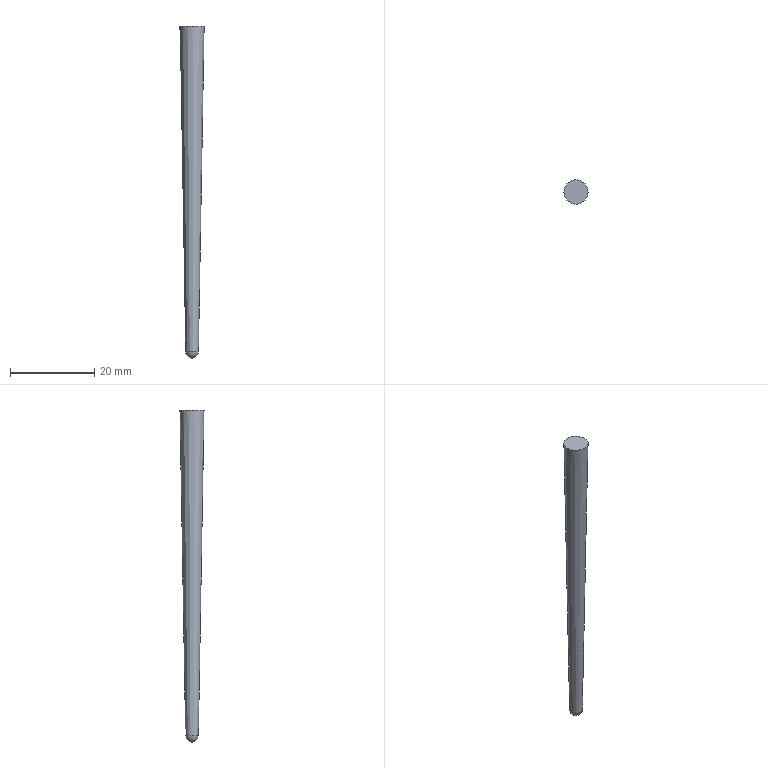Part | NX | features solid 2 | 1 solid | 4 faces | box 5.751 x 5.751 x 78.8 mm | volume 1220 mm3 | plane 2 | cone 1 | torus 1
STEP:
#1=CARTESIAN_POINT('',(-0.02595,0.,23.24));
#2=VERTEX_POINT('',#1);
#3=CARTESIAN_POINT('',(0.,0.,23.24));
#4=DIRECTION('',(0.,0.,-1.));
#5=DIRECTION('',(-1.,0.,0.));
#6=AXIS2_PLACEMENT_3D('',#3,#4,#5);
#7=CIRCLE('',#6,0.02595);
#8=EDGE_CURVE('',#2,#2,#7,.T.);
#9=ORIENTED_EDGE('',*,*,#8,.T.);
#10=EDGE_LOOP('',(#9));
#11=FACE_BOUND('',#10,.T.);
#12=CARTESIAN_POINT('',(0.,0.,23.24));
#13=DIRECTION('',(0.,0.,-1.));
#14=DIRECTION('',(-1.,0.,0.));
#15=AXIS2_PLACEMENT_3D('',#12,#13,#14);
#16=PLANE('',#15);
#17=ADVANCED_FACE('',(#11),#16,.T.);
#18=CARTESIAN_POINT('',(2.875,0.,102.04));
#19=VERTEX_POINT('',#18);
#20=CARTESIAN_POINT('',(0.,0.,102.04));
#21=DIRECTION('',(0.,0.,-1.));
#22=DIRECTION('',(1.,0.,0.));
#23=AXIS2_PLACEMENT_3D('',#20,#21,#22);
#24=CIRCLE('',#23,2.875);
#25=EDGE_CURVE('',#19,#19,#24,.T.);
#26=ORIENTED_EDGE('',*,*,#25,.F.);
#27=EDGE_LOOP('',(#26));
#28=FACE_BOUND('',#27,.T.);
#29=CARTESIAN_POINT('',(0.,0.,102.04));
#30=DIRECTION('',(0.,0.,1.));
#31=DIRECTION('',(1.,0.,0.));
#32=AXIS2_PLACEMENT_3D('',#29,#30,#31);
#33=PLANE('',#32);
#34=ADVANCED_FACE('',(#28),#33,.T.);
#35=CARTESIAN_POINT('',(-1.526,0.,24.714));
#36=VERTEX_POINT('',#35);
#37=CARTESIAN_POINT('',(0.,0.,24.714));
#38=DIRECTION('',(0.,0.,-1.));
#39=DIRECTION('',(-1.,0.,0.));
#40=AXIS2_PLACEMENT_3D('',#37,#38,#39);
#41=CIRCLE('',#40,1.526);
#42=EDGE_CURVE('',#36,#36,#41,.F.);
#43=ORIENTED_EDGE('',*,*,#42,.T.);
#44=EDGE_LOOP('',(#43));
#45=FACE_BOUND('',#44,.T.);
#46=ORIENTED_EDGE('',*,*,#25,.T.);
#47=EDGE_LOOP('',(#46));
#48=FACE_BOUND('',#47,.T.);
#49=CARTESIAN_POINT('',(0.,0.,23.24));
#50=DIRECTION('',(0.,0.,1.));
#51=DIRECTION('',(1.,0.,0.));
#52=AXIS2_PLACEMENT_3D('',#49,#50,#51);
#53=CONICAL_SURFACE('',#52,1.5,0.01745);
#54=ADVANCED_FACE('',(#45,#48),#53,.T.);
#55=ORIENTED_EDGE('',*,*,#8,.F.);
#56=EDGE_LOOP('',(#55));
#57=FACE_BOUND('',#56,.T.);
#58=ORIENTED_EDGE('',*,*,#42,.F.);
#59=EDGE_LOOP('',(#58));
#60=FACE_BOUND('',#59,.T.);
#61=CARTESIAN_POINT('',(0.,0.,24.74));
#62=DIRECTION('',(0.,0.,-1.));
#63=DIRECTION('',(-1.,0.,0.));
#64=AXIS2_PLACEMENT_3D('',#61,#62,#63);
#65=DEGENERATE_TOROIDAL_SURFACE('',#64,0.02595,1.5,.T.);
#66=ADVANCED_FACE('',(#57,#60),#65,.T.);
#67=CLOSED_SHELL('',(#17,#34,#54,#66));
#68=MANIFOLD_SOLID_BREP('',#67);
#69=(LENGTH_UNIT()NAMED_UNIT(*)SI_UNIT(.MILLI.,.METRE.));
#70=UNCERTAINTY_MEASURE_WITH_UNIT(LENGTH_MEASURE(0.00001),#69,'','');
#71=(NAMED_UNIT(*)PLANE_ANGLE_UNIT()SI_UNIT($,.RADIAN.));
#72=(NAMED_UNIT(*)SI_UNIT($,.STERADIAN.)SOLID_ANGLE_UNIT());
#73=(GEOMETRIC_REPRESENTATION_CONTEXT(3)GLOBAL_UNCERTAINTY_ASSIGNED_CONTEXT((#70))GLOBAL_UNIT_ASSIGNED_CONTEXT((#69,#71,#72))REPRESENTATION_CONTEXT('',''));
#74=ADVANCED_BREP_SHAPE_REPRESENTATION('',(#68),#73);